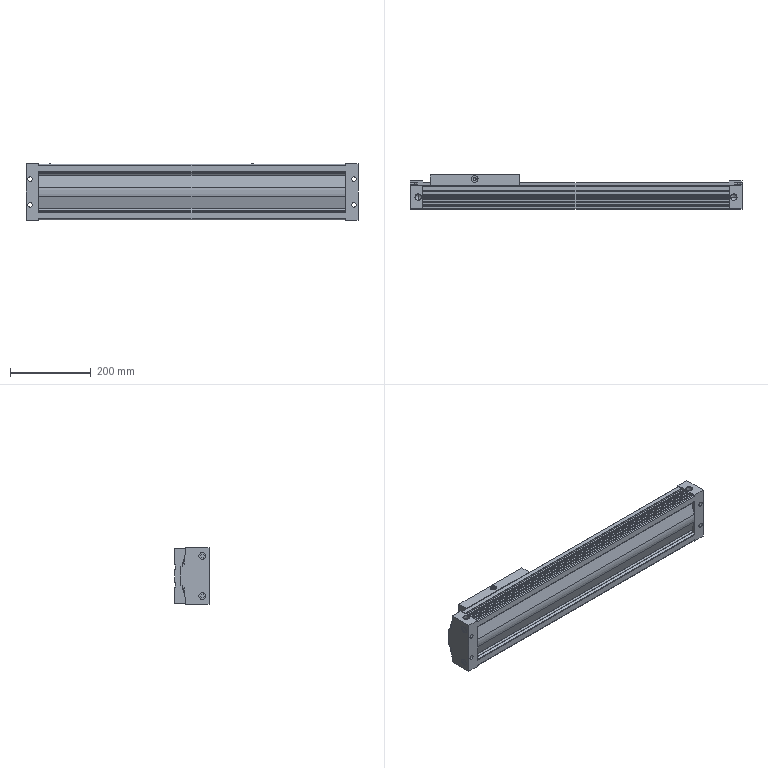Part | STEP file | 6 solids | 361 faces | box 820 x 84 x 139 mm | volume 6920085 mm3 | plane 214 | cylinder 115 | cone 32 | commonest cylinder face diameters 4 x12 6.647 x12 16.662 x12 2 x8 11 x8 2.1 x6